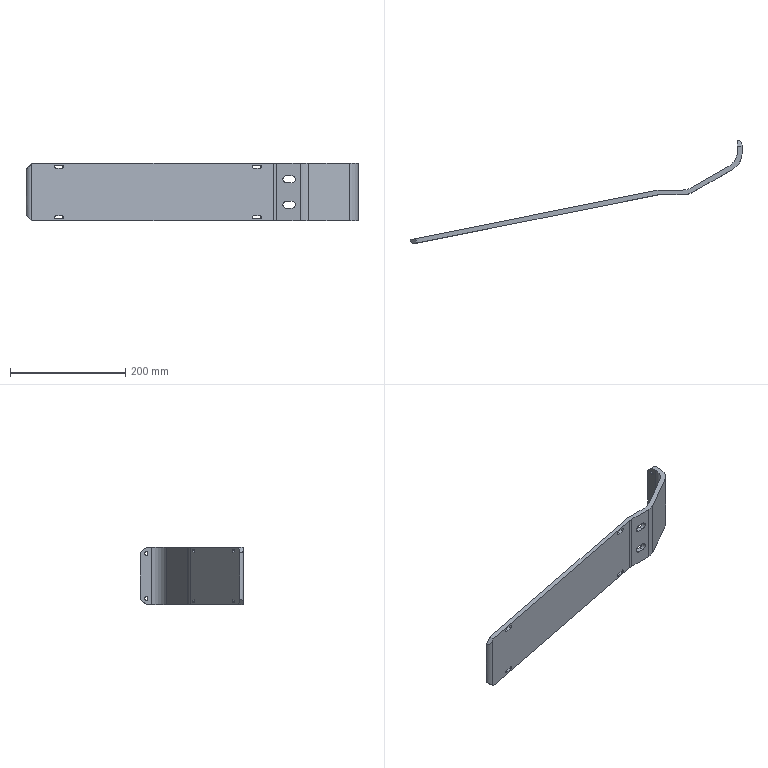Part | SolidWorks | features ICE 3, Fillet 2, Chamfer 1, ExtruThin 1 | 1 solid | 54 faces | box 576.058 x 178.723 x 100 mm | volume 494950 mm3 | cylinder 28 | plane 26 | commonest cylinder face diameters 5 x12 60 x6 6 x4 12 x4 16 x2